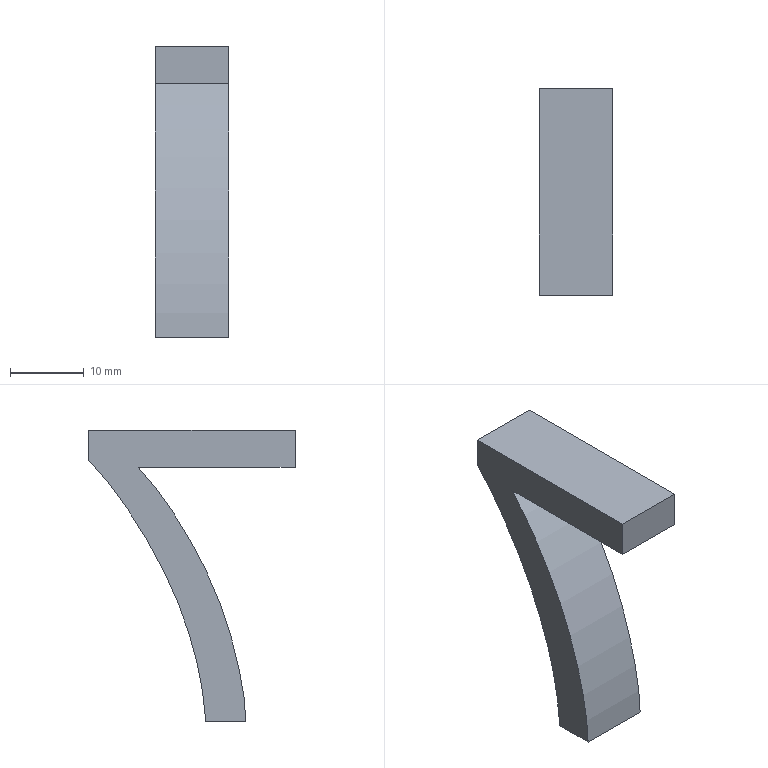Part | NX | features solid 2 | 1 solid | 9 faces | box 10 x 28.023 x 39.602 mm | volume 3381 mm3 | plane 7 | spline 2
STEP:
#1=CARTESIAN_POINT('',(2250.,-183.677,-555.446));
#2=VERTEX_POINT('',#1);
#3=CARTESIAN_POINT('',(2250.,-205.,-555.446));
#4=VERTEX_POINT('',#3);
#5=CARTESIAN_POINT('',(2250.,-183.677,-555.446));
#6=CARTESIAN_POINT('',(2250.,-190.785,-555.446));
#7=CARTESIAN_POINT('',(2250.,-197.892,-555.446));
#8=CARTESIAN_POINT('',(2250.,-205.,-555.446));
#9=B_SPLINE_CURVE_WITH_KNOTS('',3,(#5,#6,#7,#8),.UNSPECIFIED.,.F.,.F.,(4,4),(0.,0.1597),.PIECEWISE_BEZIER_KNOTS.);
#10=EDGE_CURVE('',#2,#4,#9,.T.);
#11=ORIENTED_EDGE('',*,*,#10,.F.);
#12=CARTESIAN_POINT('',(2260.,-183.677,-555.446));
#13=VERTEX_POINT('',#12);
#14=CARTESIAN_POINT('',(2260.,-183.677,-555.446));
#15=DIRECTION('',(-1.,0.,0.));
#16=VECTOR('',#15,1000.);
#17=LINE('',#14,#16);
#18=EDGE_CURVE('',#13,#2,#17,.T.);
#19=ORIENTED_EDGE('',*,*,#18,.F.);
#20=CARTESIAN_POINT('',(2260.,-205.,-555.446));
#21=VERTEX_POINT('',#20);
#22=CARTESIAN_POINT('',(2260.,-183.677,-555.446));
#23=CARTESIAN_POINT('',(2260.,-190.785,-555.446));
#24=CARTESIAN_POINT('',(2260.,-197.892,-555.446));
#25=CARTESIAN_POINT('',(2260.,-205.,-555.446));
#26=B_SPLINE_CURVE_WITH_KNOTS('',3,(#22,#23,#24,#25),.UNSPECIFIED.,.F.,.F.,(4,4),(0.,0.1597),.PIECEWISE_BEZIER_KNOTS.);
#27=EDGE_CURVE('',#13,#21,#26,.T.);
#28=ORIENTED_EDGE('',*,*,#27,.T.);
#29=CARTESIAN_POINT('',(2260.,-205.,-555.446));
#30=DIRECTION('',(-1.,0.,0.));
#31=VECTOR('',#30,1000.);
#32=LINE('',#29,#31);
#33=EDGE_CURVE('',#21,#4,#32,.T.);
#34=ORIENTED_EDGE('',*,*,#33,.T.);
#35=EDGE_LOOP('',(#11,#19,#28,#34));
#36=FACE_BOUND('',#35,.T.);
#37=CARTESIAN_POINT('',(2260.,-183.677,-555.446));
#38=DIRECTION('',(0.,0.,-1.));
#39=DIRECTION('',(-1.,0.,0.));
#40=AXIS2_PLACEMENT_3D('',#37,#38,#39);
#41=PLANE('',#40);
#42=ADVANCED_FACE('',(#36),#41,.T.);
#43=CARTESIAN_POINT('',(2250.,-205.,-550.398));
#44=VERTEX_POINT('',#43);
#45=CARTESIAN_POINT('',(2250.,-205.,-555.446));
#46=CARTESIAN_POINT('',(2250.,-205.,-553.763));
#47=CARTESIAN_POINT('',(2250.,-205.,-552.08));
#48=CARTESIAN_POINT('',(2250.,-205.,-550.398));
#49=B_SPLINE_CURVE_WITH_KNOTS('',3,(#45,#46,#47,#48),.UNSPECIFIED.,.F.,.F.,(4,4),(0.1597,0.1975),.PIECEWISE_BEZIER_KNOTS.);
#50=EDGE_CURVE('',#4,#44,#49,.T.);
#51=ORIENTED_EDGE('',*,*,#50,.F.);
#52=ORIENTED_EDGE('',*,*,#33,.F.);
#53=CARTESIAN_POINT('',(2260.,-205.,-550.398));
#54=VERTEX_POINT('',#53);
#55=CARTESIAN_POINT('',(2260.,-205.,-555.446));
#56=CARTESIAN_POINT('',(2260.,-205.,-553.763));
#57=CARTESIAN_POINT('',(2260.,-205.,-552.08));
#58=CARTESIAN_POINT('',(2260.,-205.,-550.398));
#59=B_SPLINE_CURVE_WITH_KNOTS('',3,(#55,#56,#57,#58),.UNSPECIFIED.,.F.,.F.,(4,4),(0.1597,0.1975),.PIECEWISE_BEZIER_KNOTS.);
#60=EDGE_CURVE('',#21,#54,#59,.T.);
#61=ORIENTED_EDGE('',*,*,#60,.T.);
#62=CARTESIAN_POINT('',(2260.,-205.,-550.398));
#63=DIRECTION('',(-1.,0.,0.));
#64=VECTOR('',#63,1000.);
#65=LINE('',#62,#64);
#66=EDGE_CURVE('',#54,#44,#65,.T.);
#67=ORIENTED_EDGE('',*,*,#66,.T.);
#68=EDGE_LOOP('',(#51,#52,#61,#67));
#69=FACE_BOUND('',#68,.T.);
#70=CARTESIAN_POINT('',(2260.,-205.,-555.446));
#71=DIRECTION('',(0.,-1.,0.));
#72=DIRECTION('',(1.,0.,0.));
#73=AXIS2_PLACEMENT_3D('',#70,#71,#72);
#74=PLANE('',#73);
#75=ADVANCED_FACE('',(#69),#74,.T.);
#76=CARTESIAN_POINT('',(2250.,-176.977,-550.398));
#77=VERTEX_POINT('',#76);
#78=CARTESIAN_POINT('',(2250.,-205.,-550.398));
#79=CARTESIAN_POINT('',(2250.,-195.659,-550.398));
#80=CARTESIAN_POINT('',(2250.,-186.318,-550.398));
#81=CARTESIAN_POINT('',(2250.,-176.977,-550.398));
#82=B_SPLINE_CURVE_WITH_KNOTS('',3,(#78,#79,#80,#81),.UNSPECIFIED.,.F.,.F.,(4,4),(0.1975,0.4074),.PIECEWISE_BEZIER_KNOTS.);
#83=EDGE_CURVE('',#44,#77,#82,.T.);
#84=ORIENTED_EDGE('',*,*,#83,.F.);
#85=ORIENTED_EDGE('',*,*,#66,.F.);
#86=CARTESIAN_POINT('',(2260.,-176.977,-550.398));
#87=VERTEX_POINT('',#86);
#88=CARTESIAN_POINT('',(2260.,-205.,-550.398));
#89=CARTESIAN_POINT('',(2260.,-195.659,-550.398));
#90=CARTESIAN_POINT('',(2260.,-186.318,-550.398));
#91=CARTESIAN_POINT('',(2260.,-176.977,-550.398));
#92=B_SPLINE_CURVE_WITH_KNOTS('',3,(#88,#89,#90,#91),.UNSPECIFIED.,.F.,.F.,(4,4),(0.1975,0.4074),.PIECEWISE_BEZIER_KNOTS.);
#93=EDGE_CURVE('',#54,#87,#92,.T.);
#94=ORIENTED_EDGE('',*,*,#93,.T.);
#95=CARTESIAN_POINT('',(2260.,-176.977,-550.398));
#96=DIRECTION('',(-1.,0.,0.));
#97=VECTOR('',#96,1000.);
#98=LINE('',#95,#97);
#99=EDGE_CURVE('',#87,#77,#98,.T.);
#100=ORIENTED_EDGE('',*,*,#99,.T.);
#101=EDGE_LOOP('',(#84,#85,#94,#100));
#102=FACE_BOUND('',#101,.T.);
#103=CARTESIAN_POINT('',(2260.,-205.,-550.398));
#104=DIRECTION('',(0.,0.,1.));
#105=DIRECTION('',(1.,0.,0.));
#106=AXIS2_PLACEMENT_3D('',#103,#104,#105);
#107=PLANE('',#106);
#108=ADVANCED_FACE('',(#102),#107,.T.);
#109=CARTESIAN_POINT('',(2250.,-176.977,-554.497));
#110=VERTEX_POINT('',#109);
#111=CARTESIAN_POINT('',(2250.,-176.977,-550.398));
#112=CARTESIAN_POINT('',(2250.,-176.977,-551.764));
#113=CARTESIAN_POINT('',(2250.,-176.977,-553.131));
#114=CARTESIAN_POINT('',(2250.,-176.977,-554.497));
#115=B_SPLINE_CURVE_WITH_KNOTS('',3,(#111,#112,#113,#114),.UNSPECIFIED.,.F.,.F.,(4,4),(0.4074,0.4381),.PIECEWISE_BEZIER_KNOTS.);
#116=EDGE_CURVE('',#77,#110,#115,.T.);
#117=ORIENTED_EDGE('',*,*,#116,.F.);
#118=ORIENTED_EDGE('',*,*,#99,.F.);
#119=CARTESIAN_POINT('',(2260.,-176.977,-554.497));
#120=VERTEX_POINT('',#119);
#121=CARTESIAN_POINT('',(2260.,-176.977,-550.398));
#122=CARTESIAN_POINT('',(2260.,-176.977,-551.764));
#123=CARTESIAN_POINT('',(2260.,-176.977,-553.131));
#124=CARTESIAN_POINT('',(2260.,-176.977,-554.497));
#125=B_SPLINE_CURVE_WITH_KNOTS('',3,(#121,#122,#123,#124),.UNSPECIFIED.,.F.,.F.,(4,4),(0.4074,0.4381),.PIECEWISE_BEZIER_KNOTS.);
#126=EDGE_CURVE('',#87,#120,#125,.T.);
#127=ORIENTED_EDGE('',*,*,#126,.T.);
#128=CARTESIAN_POINT('',(2260.,-176.977,-554.497));
#129=DIRECTION('',(-1.,0.,0.));
#130=VECTOR('',#129,1000.);
#131=LINE('',#128,#130);
#132=EDGE_CURVE('',#120,#110,#131,.T.);
#133=ORIENTED_EDGE('',*,*,#132,.T.);
#134=EDGE_LOOP('',(#117,#118,#127,#133));
#135=FACE_BOUND('',#134,.T.);
#136=CARTESIAN_POINT('',(2260.,-176.977,-550.398));
#137=DIRECTION('',(0.,1.,0.));
#138=DIRECTION('',(-1.,0.,0.));
#139=AXIS2_PLACEMENT_3D('',#136,#137,#138);
#140=PLANE('',#139);
#141=ADVANCED_FACE('',(#135),#140,.T.);
#142=CARTESIAN_POINT('',(2250.,-192.87,-590.));
#143=VERTEX_POINT('',#142);
#144=CARTESIAN_POINT('',(2250.,-176.977,-554.497));
#145=CARTESIAN_POINT('',(2250.,-179.639,-557.266));
#146=CARTESIAN_POINT('',(2250.,-182.254,-560.86));
#147=CARTESIAN_POINT('',(2250.,-187.492,-569.774));
#148=CARTESIAN_POINT('',(2250.,-189.505,-574.367));
#149=CARTESIAN_POINT('',(2250.,-191.915,-582.435));
#150=CARTESIAN_POINT('',(2250.,-192.579,-586.069));
#151=CARTESIAN_POINT('',(2250.,-192.87,-590.));
#152=B_SPLINE_CURVE_WITH_KNOTS('',3,(#144,#145,#146,#147,#148,#149,#150,#151),.UNSPECIFIED.,.F.,.F.,(4,2,2,4),(0.4381,0.5386,0.6394,0.7112),.UNSPECIFIED.);
#153=EDGE_CURVE('',#110,#143,#152,.T.);
#154=ORIENTED_EDGE('',*,*,#153,.F.);
#155=ORIENTED_EDGE('',*,*,#132,.F.);
#156=CARTESIAN_POINT('',(2260.,-192.87,-590.));
#157=VERTEX_POINT('',#156);
#158=CARTESIAN_POINT('',(2260.,-176.977,-554.497));
#159=CARTESIAN_POINT('',(2260.,-179.639,-557.266));
#160=CARTESIAN_POINT('',(2260.,-182.254,-560.86));
#161=CARTESIAN_POINT('',(2260.,-187.492,-569.774));
#162=CARTESIAN_POINT('',(2260.,-189.505,-574.367));
#163=CARTESIAN_POINT('',(2260.,-191.915,-582.435));
#164=CARTESIAN_POINT('',(2260.,-192.579,-586.069));
#165=CARTESIAN_POINT('',(2260.,-192.87,-590.));
#166=B_SPLINE_CURVE_WITH_KNOTS('',3,(#158,#159,#160,#161,#162,#163,#164,#165),.UNSPECIFIED.,.F.,.F.,(4,2,2,4),(0.4381,0.5386,0.6394,0.7112),.UNSPECIFIED.);
#167=EDGE_CURVE('',#120,#157,#166,.T.);
#168=ORIENTED_EDGE('',*,*,#167,.T.);
#169=CARTESIAN_POINT('',(2260.,-192.87,-590.));
#170=DIRECTION('',(-1.,0.,0.));
#171=VECTOR('',#170,1000.);
#172=LINE('',#169,#171);
#173=EDGE_CURVE('',#157,#143,#172,.T.);
#174=ORIENTED_EDGE('',*,*,#173,.T.);
#175=EDGE_LOOP('',(#154,#155,#168,#174));
#176=FACE_BOUND('',#175,.T.);
#177=CARTESIAN_POINT('',(2260.,-176.977,-554.497));
#178=CARTESIAN_POINT('',(2250.,-176.977,-554.497));
#179=CARTESIAN_POINT('',(2260.,-178.785,-556.378));
#180=CARTESIAN_POINT('',(2250.,-178.785,-556.378));
#181=CARTESIAN_POINT('',(2260.,-182.332,-560.872));
#182=CARTESIAN_POINT('',(2250.,-182.332,-560.872));
#183=CARTESIAN_POINT('',(2260.,-186.863,-568.587));
#184=CARTESIAN_POINT('',(2250.,-186.863,-568.587));
#185=CARTESIAN_POINT('',(2260.,-189.528,-574.811));
#186=CARTESIAN_POINT('',(2250.,-189.528,-574.811));
#187=CARTESIAN_POINT('',(2260.,-191.668,-581.096));
#188=CARTESIAN_POINT('',(2250.,-191.668,-581.096));
#189=CARTESIAN_POINT('',(2260.,-192.594,-586.262));
#190=CARTESIAN_POINT('',(2250.,-192.594,-586.262));
#191=CARTESIAN_POINT('',(2260.,-192.87,-590.));
#192=CARTESIAN_POINT('',(2250.,-192.87,-590.));
#193=B_SPLINE_SURFACE_WITH_KNOTS('',3,1,((#177,#178),(#179,#180),(#181,#182),(#183,#184),(#185,#186),(#187,#188),(#189,#190),(#191,#192)),.SURF_OF_LINEAR_EXTRUSION.,.F.,.F.,.F.,(4,1,1,1,1,4),(2,2),(0.4381,0.5064,0.5746,0.6088,0.6429,0.7112),(0.,1.),.UNSPECIFIED.);
#194=ADVANCED_FACE('',(#176),#193,.T.);
#195=CARTESIAN_POINT('',(2250.,-198.315,-590.));
#196=VERTEX_POINT('',#195);
#197=CARTESIAN_POINT('',(2250.,-192.87,-590.));
#198=CARTESIAN_POINT('',(2250.,-194.685,-590.));
#199=CARTESIAN_POINT('',(2250.,-196.5,-590.));
#200=CARTESIAN_POINT('',(2250.,-198.315,-590.));
#201=B_SPLINE_CURVE_WITH_KNOTS('',3,(#197,#198,#199,#200),.UNSPECIFIED.,.F.,.F.,(4,4),(0.7112,0.7506),.PIECEWISE_BEZIER_KNOTS.);
#202=EDGE_CURVE('',#143,#196,#201,.T.);
#203=ORIENTED_EDGE('',*,*,#202,.F.);
#204=ORIENTED_EDGE('',*,*,#173,.F.);
#205=CARTESIAN_POINT('',(2260.,-198.315,-590.));
#206=VERTEX_POINT('',#205);
#207=CARTESIAN_POINT('',(2260.,-192.87,-590.));
#208=CARTESIAN_POINT('',(2260.,-194.685,-590.));
#209=CARTESIAN_POINT('',(2260.,-196.5,-590.));
#210=CARTESIAN_POINT('',(2260.,-198.315,-590.));
#211=B_SPLINE_CURVE_WITH_KNOTS('',3,(#207,#208,#209,#210),.UNSPECIFIED.,.F.,.F.,(4,4),(0.7112,0.7506),.PIECEWISE_BEZIER_KNOTS.);
#212=EDGE_CURVE('',#157,#206,#211,.T.);
#213=ORIENTED_EDGE('',*,*,#212,.T.);
#214=CARTESIAN_POINT('',(2260.,-198.315,-590.));
#215=DIRECTION('',(-1.,0.,0.));
#216=VECTOR('',#215,1000.);
#217=LINE('',#214,#216);
#218=EDGE_CURVE('',#206,#196,#217,.T.);
#219=ORIENTED_EDGE('',*,*,#218,.T.);
#220=EDGE_LOOP('',(#203,#204,#213,#219));
#221=FACE_BOUND('',#220,.T.);
#222=CARTESIAN_POINT('',(2260.,-192.87,-590.));
#223=DIRECTION('',(0.,0.,-1.));
#224=DIRECTION('',(0.,1.,0.));
#225=AXIS2_PLACEMENT_3D('',#222,#223,#224);
#226=PLANE('',#225);
#227=ADVANCED_FACE('',(#221),#226,.T.);
#228=CARTESIAN_POINT('',(2250.,-198.315,-590.));
#229=CARTESIAN_POINT('',(2250.,-198.254,-586.895));
#230=CARTESIAN_POINT('',(2250.,-197.612,-583.132));
#231=CARTESIAN_POINT('',(2250.,-195.137,-574.27));
#232=CARTESIAN_POINT('',(2250.,-193.344,-570.008));
#233=CARTESIAN_POINT('',(2250.,-188.765,-561.764));
#234=CARTESIAN_POINT('',(2250.,-186.293,-558.306));
#235=CARTESIAN_POINT('',(2250.,-183.677,-555.446));
#236=B_SPLINE_CURVE_WITH_KNOTS('',3,(#228,#229,#230,#231,#232,#233,#234,#235),.UNSPECIFIED.,.F.,.F.,(4,2,2,4),(0.7506,0.834,0.9172,1.),.UNSPECIFIED.);
#237=EDGE_CURVE('',#196,#2,#236,.T.);
#238=ORIENTED_EDGE('',*,*,#237,.F.);
#239=ORIENTED_EDGE('',*,*,#218,.F.);
#240=CARTESIAN_POINT('',(2260.,-198.315,-590.));
#241=CARTESIAN_POINT('',(2260.,-198.254,-586.895));
#242=CARTESIAN_POINT('',(2260.,-197.612,-583.132));
#243=CARTESIAN_POINT('',(2260.,-195.137,-574.27));
#244=CARTESIAN_POINT('',(2260.,-193.344,-570.008));
#245=CARTESIAN_POINT('',(2260.,-188.765,-561.764));
#246=CARTESIAN_POINT('',(2260.,-186.293,-558.306));
#247=CARTESIAN_POINT('',(2260.,-183.677,-555.446));
#248=B_SPLINE_CURVE_WITH_KNOTS('',3,(#240,#241,#242,#243,#244,#245,#246,#247),.UNSPECIFIED.,.F.,.F.,(4,2,2,4),(0.7506,0.834,0.9172,1.),.UNSPECIFIED.);
#249=EDGE_CURVE('',#206,#13,#248,.T.);
#250=ORIENTED_EDGE('',*,*,#249,.T.);
#251=ORIENTED_EDGE('',*,*,#18,.T.);
#252=EDGE_LOOP('',(#238,#239,#250,#251));
#253=FACE_BOUND('',#252,.T.);
#254=CARTESIAN_POINT('',(2260.,-198.315,-590.));
#255=CARTESIAN_POINT('',(2250.,-198.315,-590.));
#256=CARTESIAN_POINT('',(2260.,-198.27,-587.678));
#257=CARTESIAN_POINT('',(2250.,-198.27,-587.678));
#258=CARTESIAN_POINT('',(2260.,-197.716,-583.686));
#259=CARTESIAN_POINT('',(2250.,-197.716,-583.686));
#260=CARTESIAN_POINT('',(2260.,-195.973,-577.068));
#261=CARTESIAN_POINT('',(2250.,-195.973,-577.068));
#262=CARTESIAN_POINT('',(2260.,-194.2,-572.195));
#263=CARTESIAN_POINT('',(2250.,-194.2,-572.195));
#264=CARTESIAN_POINT('',(2260.,-191.978,-567.453));
#265=CARTESIAN_POINT('',(2250.,-191.978,-567.453));
#266=CARTESIAN_POINT('',(2260.,-188.46,-561.308));
#267=CARTESIAN_POINT('',(2250.,-188.46,-561.308));
#268=CARTESIAN_POINT('',(2260.,-185.645,-557.598));
#269=CARTESIAN_POINT('',(2250.,-185.645,-557.598));
#270=CARTESIAN_POINT('',(2260.,-183.677,-555.446));
#271=CARTESIAN_POINT('',(2250.,-183.677,-555.446));
#272=B_SPLINE_SURFACE_WITH_KNOTS('',3,1,((#254,#255),(#256,#257),(#258,#259),(#260,#261),(#262,#263),(#264,#265),(#266,#267),(#268,#269),(#270,#271)),.SURF_OF_LINEAR_EXTRUSION.,.F.,.F.,.F.,(4,1,1,1,1,1,4),(2,2),(0.7506,0.813,0.8442,0.8753,0.9065,0.9377,1.),(0.,1.),.UNSPECIFIED.);
#273=ADVANCED_FACE('',(#253),#272,.T.);
#274=ORIENTED_EDGE('',*,*,#27,.F.);
#275=ORIENTED_EDGE('',*,*,#249,.F.);
#276=ORIENTED_EDGE('',*,*,#212,.F.);
#277=ORIENTED_EDGE('',*,*,#167,.F.);
#278=ORIENTED_EDGE('',*,*,#126,.F.);
#279=ORIENTED_EDGE('',*,*,#93,.F.);
#280=ORIENTED_EDGE('',*,*,#60,.F.);
#281=EDGE_LOOP('',(#274,#275,#276,#277,#278,#279,#280));
#282=FACE_BOUND('',#281,.T.);
#283=CARTESIAN_POINT('',(2260.,-187.449,-570.147));
#284=DIRECTION('',(-1.,0.,0.));
#285=DIRECTION('',(0.,-1.,0.));
#286=AXIS2_PLACEMENT_3D('',#283,#284,#285);
#287=PLANE('',#286);
#288=ADVANCED_FACE('',(#282),#287,.F.);
#289=ORIENTED_EDGE('',*,*,#10,.T.);
#290=ORIENTED_EDGE('',*,*,#50,.T.);
#291=ORIENTED_EDGE('',*,*,#83,.T.);
#292=ORIENTED_EDGE('',*,*,#116,.T.);
#293=ORIENTED_EDGE('',*,*,#153,.T.);
#294=ORIENTED_EDGE('',*,*,#202,.T.);
#295=ORIENTED_EDGE('',*,*,#237,.T.);
#296=EDGE_LOOP('',(#289,#290,#291,#292,#293,#294,#295));
#297=FACE_BOUND('',#296,.T.);
#298=CARTESIAN_POINT('',(2250.,-187.449,-570.147));
#299=DIRECTION('',(-1.,0.,0.));
#300=DIRECTION('',(0.,-1.,0.));
#301=AXIS2_PLACEMENT_3D('',#298,#299,#300);
#302=PLANE('',#301);
#303=ADVANCED_FACE('',(#297),#302,.T.);
#304=CLOSED_SHELL('',(#42,#75,#108,#141,#194,#227,#273,#288,#303));
#305=MANIFOLD_SOLID_BREP('',#304);
#306=(LENGTH_UNIT()NAMED_UNIT(*)SI_UNIT(.MILLI.,.METRE.));
#307=UNCERTAINTY_MEASURE_WITH_UNIT(LENGTH_MEASURE(0.0508),#306,'','');
#308=(NAMED_UNIT(*)PLANE_ANGLE_UNIT()SI_UNIT($,.RADIAN.));
#309=(NAMED_UNIT(*)SI_UNIT($,.STERADIAN.)SOLID_ANGLE_UNIT());
#310=(GEOMETRIC_REPRESENTATION_CONTEXT(3)GLOBAL_UNCERTAINTY_ASSIGNED_CONTEXT((#307))GLOBAL_UNIT_ASSIGNED_CONTEXT((#306,#308,#309))REPRESENTATION_CONTEXT('',''));
#311=ADVANCED_BREP_SHAPE_REPRESENTATION('',(#305),#310);